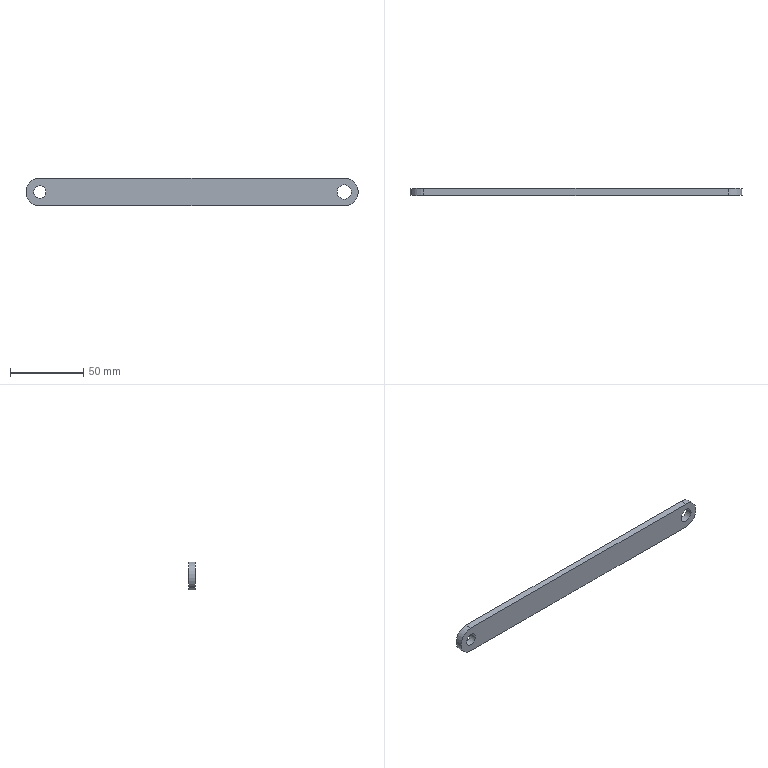Part | NX | features BREP 1 | 1 solid | 10 faces | box 227.013 x 4.763 x 19.05 mm | volume 19604 mm3 | cylinder 6 | plane 4 | commonest cylinder face diameters 8.382 x2 9.779 x2 19.05 x2
STEP:
#1=CARTESIAN_POINT('',(-103.981,0.,9.525));
#2=VERTEX_POINT('',#1);
#3=CARTESIAN_POINT('',(103.981,0.,9.525));
#4=VERTEX_POINT('',#3);
#5=CARTESIAN_POINT('',(-103.981,0.,9.525));
#6=DIRECTION('',(1.,0.,0.));
#7=VECTOR('',#6,1000.);
#8=LINE('',#5,#7);
#9=EDGE_CURVE('',#2,#4,#8,.T.);
#10=ORIENTED_EDGE('',*,*,#9,.T.);
#11=CARTESIAN_POINT('',(103.981,0.,-9.525));
#12=VERTEX_POINT('',#11);
#13=CARTESIAN_POINT('',(103.981,0.,0.));
#14=DIRECTION('',(0.,1.,0.));
#15=DIRECTION('',(0.,0.,1.));
#16=AXIS2_PLACEMENT_3D('',#13,#14,#15);
#17=CIRCLE('',#16,9.525);
#18=EDGE_CURVE('',#4,#12,#17,.T.);
#19=ORIENTED_EDGE('',*,*,#18,.T.);
#20=CARTESIAN_POINT('',(-103.981,0.,-9.525));
#21=VERTEX_POINT('',#20);
#22=CARTESIAN_POINT('',(103.981,0.,-9.525));
#23=DIRECTION('',(-1.,0.,0.));
#24=VECTOR('',#23,1000.);
#25=LINE('',#22,#24);
#26=EDGE_CURVE('',#12,#21,#25,.T.);
#27=ORIENTED_EDGE('',*,*,#26,.T.);
#28=CARTESIAN_POINT('',(-103.981,0.,0.));
#29=DIRECTION('',(0.,1.,0.));
#30=DIRECTION('',(0.,0.,-1.));
#31=AXIS2_PLACEMENT_3D('',#28,#29,#30);
#32=CIRCLE('',#31,9.525);
#33=EDGE_CURVE('',#21,#2,#32,.T.);
#34=ORIENTED_EDGE('',*,*,#33,.T.);
#35=EDGE_LOOP('',(#10,#19,#27,#34));
#36=FACE_BOUND('',#35,.T.);
#37=CARTESIAN_POINT('',(99.092,0.,0.));
#38=VERTEX_POINT('',#37);
#39=CARTESIAN_POINT('',(108.871,0.,0.));
#40=VERTEX_POINT('',#39);
#41=CARTESIAN_POINT('',(103.981,0.,0.));
#42=DIRECTION('',(0.,-1.,0.));
#43=DIRECTION('',(-1.,0.,0.));
#44=AXIS2_PLACEMENT_3D('',#41,#42,#43);
#45=CIRCLE('',#44,4.89);
#46=EDGE_CURVE('',#38,#40,#45,.T.);
#47=ORIENTED_EDGE('',*,*,#46,.T.);
#48=CARTESIAN_POINT('',(103.981,0.,0.));
#49=DIRECTION('',(0.,-1.,0.));
#50=DIRECTION('',(1.,0.,0.));
#51=AXIS2_PLACEMENT_3D('',#48,#49,#50);
#52=CIRCLE('',#51,4.89);
#53=EDGE_CURVE('',#40,#38,#52,.T.);
#54=ORIENTED_EDGE('',*,*,#53,.T.);
#55=EDGE_LOOP('',(#47,#54));
#56=FACE_BOUND('',#55,.T.);
#57=CARTESIAN_POINT('',(-108.172,0.,0.));
#58=VERTEX_POINT('',#57);
#59=CARTESIAN_POINT('',(-99.79,0.,0.));
#60=VERTEX_POINT('',#59);
#61=CARTESIAN_POINT('',(-103.981,0.,0.));
#62=DIRECTION('',(0.,-1.,0.));
#63=DIRECTION('',(-1.,0.,0.));
#64=AXIS2_PLACEMENT_3D('',#61,#62,#63);
#65=CIRCLE('',#64,4.191);
#66=EDGE_CURVE('',#58,#60,#65,.T.);
#67=ORIENTED_EDGE('',*,*,#66,.T.);
#68=CARTESIAN_POINT('',(-103.981,0.,0.));
#69=DIRECTION('',(0.,-1.,0.));
#70=DIRECTION('',(1.,0.,0.));
#71=AXIS2_PLACEMENT_3D('',#68,#69,#70);
#72=CIRCLE('',#71,4.191);
#73=EDGE_CURVE('',#60,#58,#72,.T.);
#74=ORIENTED_EDGE('',*,*,#73,.T.);
#75=EDGE_LOOP('',(#67,#74));
#76=FACE_BOUND('',#75,.T.);
#77=CARTESIAN_POINT('',(0.,0.,0.));
#78=DIRECTION('',(0.,1.,0.));
#79=DIRECTION('',(1.,0.,0.));
#80=AXIS2_PLACEMENT_3D('',#77,#78,#79);
#81=PLANE('',#80);
#82=ADVANCED_FACE('',(#36,#56,#76),#81,.T.);
#83=CARTESIAN_POINT('',(-103.981,-4.763,-9.525));
#84=VERTEX_POINT('',#83);
#85=CARTESIAN_POINT('',(-103.981,0.,-9.525));
#86=DIRECTION('',(0.,-1.,0.));
#87=VECTOR('',#86,1000.);
#88=LINE('',#85,#87);
#89=EDGE_CURVE('',#21,#84,#88,.T.);
#90=ORIENTED_EDGE('',*,*,#89,.T.);
#91=CARTESIAN_POINT('',(-103.981,-4.763,9.525));
#92=VERTEX_POINT('',#91);
#93=CARTESIAN_POINT('',(-103.981,-4.763,0.));
#94=DIRECTION('',(0.,1.,0.));
#95=DIRECTION('',(0.,0.,-1.));
#96=AXIS2_PLACEMENT_3D('',#93,#94,#95);
#97=CIRCLE('',#96,9.525);
#98=EDGE_CURVE('',#84,#92,#97,.T.);
#99=ORIENTED_EDGE('',*,*,#98,.T.);
#100=CARTESIAN_POINT('',(-103.981,0.,9.525));
#101=DIRECTION('',(0.,-1.,0.));
#102=VECTOR('',#101,1000.);
#103=LINE('',#100,#102);
#104=EDGE_CURVE('',#2,#92,#103,.T.);
#105=ORIENTED_EDGE('',*,*,#104,.F.);
#106=ORIENTED_EDGE('',*,*,#33,.F.);
#107=EDGE_LOOP('',(#90,#99,#105,#106));
#108=FACE_BOUND('',#107,.T.);
#109=CARTESIAN_POINT('',(-103.981,-2.381,0.));
#110=DIRECTION('',(0.,1.,0.));
#111=DIRECTION('',(0.,0.,-1.));
#112=AXIS2_PLACEMENT_3D('',#109,#110,#111);
#113=CYLINDRICAL_SURFACE('',#112,9.525);
#114=ADVANCED_FACE('',(#108),#113,.T.);
#115=ORIENTED_EDGE('',*,*,#104,.T.);
#116=CARTESIAN_POINT('',(103.981,-4.763,9.525));
#117=VERTEX_POINT('',#116);
#118=CARTESIAN_POINT('',(-103.981,-4.763,9.525));
#119=DIRECTION('',(1.,0.,0.));
#120=VECTOR('',#119,1000.);
#121=LINE('',#118,#120);
#122=EDGE_CURVE('',#92,#117,#121,.T.);
#123=ORIENTED_EDGE('',*,*,#122,.T.);
#124=CARTESIAN_POINT('',(103.981,0.,9.525));
#125=DIRECTION('',(0.,-1.,0.));
#126=VECTOR('',#125,1000.);
#127=LINE('',#124,#126);
#128=EDGE_CURVE('',#4,#117,#127,.T.);
#129=ORIENTED_EDGE('',*,*,#128,.F.);
#130=ORIENTED_EDGE('',*,*,#9,.F.);
#131=EDGE_LOOP('',(#115,#123,#129,#130));
#132=FACE_BOUND('',#131,.T.);
#133=CARTESIAN_POINT('',(0.,-2.381,9.525));
#134=DIRECTION('',(0.,0.,1.));
#135=DIRECTION('',(1.,0.,0.));
#136=AXIS2_PLACEMENT_3D('',#133,#134,#135);
#137=PLANE('',#136);
#138=ADVANCED_FACE('',(#132),#137,.T.);
#139=ORIENTED_EDGE('',*,*,#128,.T.);
#140=CARTESIAN_POINT('',(103.981,-4.763,-9.525));
#141=VERTEX_POINT('',#140);
#142=CARTESIAN_POINT('',(103.981,-4.763,0.));
#143=DIRECTION('',(0.,1.,0.));
#144=DIRECTION('',(0.,0.,1.));
#145=AXIS2_PLACEMENT_3D('',#142,#143,#144);
#146=CIRCLE('',#145,9.525);
#147=EDGE_CURVE('',#117,#141,#146,.T.);
#148=ORIENTED_EDGE('',*,*,#147,.T.);
#149=CARTESIAN_POINT('',(103.981,0.,-9.525));
#150=DIRECTION('',(0.,-1.,0.));
#151=VECTOR('',#150,1000.);
#152=LINE('',#149,#151);
#153=EDGE_CURVE('',#12,#141,#152,.T.);
#154=ORIENTED_EDGE('',*,*,#153,.F.);
#155=ORIENTED_EDGE('',*,*,#18,.F.);
#156=EDGE_LOOP('',(#139,#148,#154,#155));
#157=FACE_BOUND('',#156,.T.);
#158=CARTESIAN_POINT('',(103.981,-2.381,0.));
#159=DIRECTION('',(0.,1.,0.));
#160=DIRECTION('',(0.,0.,1.));
#161=AXIS2_PLACEMENT_3D('',#158,#159,#160);
#162=CYLINDRICAL_SURFACE('',#161,9.525);
#163=ADVANCED_FACE('',(#157),#162,.T.);
#164=ORIENTED_EDGE('',*,*,#153,.T.);
#165=CARTESIAN_POINT('',(103.981,-4.763,-9.525));
#166=DIRECTION('',(-1.,0.,0.));
#167=VECTOR('',#166,1000.);
#168=LINE('',#165,#167);
#169=EDGE_CURVE('',#141,#84,#168,.T.);
#170=ORIENTED_EDGE('',*,*,#169,.T.);
#171=ORIENTED_EDGE('',*,*,#89,.F.);
#172=ORIENTED_EDGE('',*,*,#26,.F.);
#173=EDGE_LOOP('',(#164,#170,#171,#172));
#174=FACE_BOUND('',#173,.T.);
#175=CARTESIAN_POINT('',(0.,-2.381,-9.525));
#176=DIRECTION('',(0.,0.,-1.));
#177=DIRECTION('',(0.,-1.,0.));
#178=AXIS2_PLACEMENT_3D('',#175,#176,#177);
#179=PLANE('',#178);
#180=ADVANCED_FACE('',(#174),#179,.T.);
#181=ORIENTED_EDGE('',*,*,#169,.F.);
#182=ORIENTED_EDGE('',*,*,#147,.F.);
#183=ORIENTED_EDGE('',*,*,#122,.F.);
#184=ORIENTED_EDGE('',*,*,#98,.F.);
#185=EDGE_LOOP('',(#181,#182,#183,#184));
#186=FACE_BOUND('',#185,.T.);
#187=CARTESIAN_POINT('',(99.092,-4.763,0.));
#188=VERTEX_POINT('',#187);
#189=CARTESIAN_POINT('',(108.871,-4.763,0.));
#190=VERTEX_POINT('',#189);
#191=CARTESIAN_POINT('',(103.981,-4.763,0.));
#192=DIRECTION('',(0.,-1.,0.));
#193=DIRECTION('',(-1.,0.,0.));
#194=AXIS2_PLACEMENT_3D('',#191,#192,#193);
#195=CIRCLE('',#194,4.89);
#196=EDGE_CURVE('',#188,#190,#195,.T.);
#197=ORIENTED_EDGE('',*,*,#196,.F.);
#198=CARTESIAN_POINT('',(103.981,-4.763,0.));
#199=DIRECTION('',(0.,-1.,0.));
#200=DIRECTION('',(1.,0.,0.));
#201=AXIS2_PLACEMENT_3D('',#198,#199,#200);
#202=CIRCLE('',#201,4.89);
#203=EDGE_CURVE('',#190,#188,#202,.T.);
#204=ORIENTED_EDGE('',*,*,#203,.F.);
#205=EDGE_LOOP('',(#197,#204));
#206=FACE_BOUND('',#205,.T.);
#207=CARTESIAN_POINT('',(-108.172,-4.763,0.));
#208=VERTEX_POINT('',#207);
#209=CARTESIAN_POINT('',(-99.79,-4.763,0.));
#210=VERTEX_POINT('',#209);
#211=CARTESIAN_POINT('',(-103.981,-4.763,0.));
#212=DIRECTION('',(0.,-1.,0.));
#213=DIRECTION('',(-1.,0.,0.));
#214=AXIS2_PLACEMENT_3D('',#211,#212,#213);
#215=CIRCLE('',#214,4.191);
#216=EDGE_CURVE('',#208,#210,#215,.T.);
#217=ORIENTED_EDGE('',*,*,#216,.F.);
#218=CARTESIAN_POINT('',(-103.981,-4.763,0.));
#219=DIRECTION('',(0.,-1.,0.));
#220=DIRECTION('',(1.,0.,0.));
#221=AXIS2_PLACEMENT_3D('',#218,#219,#220);
#222=CIRCLE('',#221,4.191);
#223=EDGE_CURVE('',#210,#208,#222,.T.);
#224=ORIENTED_EDGE('',*,*,#223,.F.);
#225=EDGE_LOOP('',(#217,#224));
#226=FACE_BOUND('',#225,.T.);
#227=CARTESIAN_POINT('',(0.,-4.763,0.));
#228=DIRECTION('',(0.,1.,0.));
#229=DIRECTION('',(1.,0.,0.));
#230=AXIS2_PLACEMENT_3D('',#227,#228,#229);
#231=PLANE('',#230);
#232=ADVANCED_FACE('',(#186,#206,#226),#231,.F.);
#233=CARTESIAN_POINT('',(108.871,0.,0.));
#234=DIRECTION('',(0.,-1.,0.));
#235=VECTOR('',#234,1000.);
#236=LINE('',#233,#235);
#237=EDGE_CURVE('',#190,#40,#236,.F.);
#238=ORIENTED_EDGE('',*,*,#237,.F.);
#239=ORIENTED_EDGE('',*,*,#203,.T.);
#240=CARTESIAN_POINT('',(99.092,0.,0.));
#241=DIRECTION('',(0.,-1.,0.));
#242=VECTOR('',#241,1000.);
#243=LINE('',#240,#242);
#244=EDGE_CURVE('',#188,#38,#243,.F.);
#245=ORIENTED_EDGE('',*,*,#244,.T.);
#246=ORIENTED_EDGE('',*,*,#53,.F.);
#247=EDGE_LOOP('',(#238,#239,#245,#246));
#248=FACE_BOUND('',#247,.T.);
#249=CARTESIAN_POINT('',(103.981,0.,0.));
#250=DIRECTION('',(0.,-1.,0.));
#251=DIRECTION('',(1.,0.,0.));
#252=AXIS2_PLACEMENT_3D('',#249,#250,#251);
#253=CYLINDRICAL_SURFACE('',#252,4.89);
#254=ADVANCED_FACE('',(#248),#253,.F.);
#255=ORIENTED_EDGE('',*,*,#244,.F.);
#256=ORIENTED_EDGE('',*,*,#196,.T.);
#257=ORIENTED_EDGE('',*,*,#237,.T.);
#258=ORIENTED_EDGE('',*,*,#46,.F.);
#259=EDGE_LOOP('',(#255,#256,#257,#258));
#260=FACE_BOUND('',#259,.T.);
#261=CARTESIAN_POINT('',(103.981,0.,0.));
#262=DIRECTION('',(0.,-1.,0.));
#263=DIRECTION('',(1.,0.,0.));
#264=AXIS2_PLACEMENT_3D('',#261,#262,#263);
#265=CYLINDRICAL_SURFACE('',#264,4.89);
#266=ADVANCED_FACE('',(#260),#265,.F.);
#267=CARTESIAN_POINT('',(-99.79,0.,0.));
#268=DIRECTION('',(0.,-1.,0.));
#269=VECTOR('',#268,1000.);
#270=LINE('',#267,#269);
#271=EDGE_CURVE('',#210,#60,#270,.F.);
#272=ORIENTED_EDGE('',*,*,#271,.F.);
#273=ORIENTED_EDGE('',*,*,#223,.T.);
#274=CARTESIAN_POINT('',(-108.172,0.,0.));
#275=DIRECTION('',(0.,-1.,0.));
#276=VECTOR('',#275,1000.);
#277=LINE('',#274,#276);
#278=EDGE_CURVE('',#208,#58,#277,.F.);
#279=ORIENTED_EDGE('',*,*,#278,.T.);
#280=ORIENTED_EDGE('',*,*,#73,.F.);
#281=EDGE_LOOP('',(#272,#273,#279,#280));
#282=FACE_BOUND('',#281,.T.);
#283=CARTESIAN_POINT('',(-103.981,0.,0.));
#284=DIRECTION('',(0.,-1.,0.));
#285=DIRECTION('',(1.,0.,0.));
#286=AXIS2_PLACEMENT_3D('',#283,#284,#285);
#287=CYLINDRICAL_SURFACE('',#286,4.191);
#288=ADVANCED_FACE('',(#282),#287,.F.);
#289=ORIENTED_EDGE('',*,*,#278,.F.);
#290=ORIENTED_EDGE('',*,*,#216,.T.);
#291=ORIENTED_EDGE('',*,*,#271,.T.);
#292=ORIENTED_EDGE('',*,*,#66,.F.);
#293=EDGE_LOOP('',(#289,#290,#291,#292));
#294=FACE_BOUND('',#293,.T.);
#295=CARTESIAN_POINT('',(-103.981,0.,0.));
#296=DIRECTION('',(0.,-1.,0.));
#297=DIRECTION('',(1.,0.,0.));
#298=AXIS2_PLACEMENT_3D('',#295,#296,#297);
#299=CYLINDRICAL_SURFACE('',#298,4.191);
#300=ADVANCED_FACE('',(#294),#299,.F.);
#301=CLOSED_SHELL('',(#82,#114,#138,#163,#180,#232,#254,#266,#288,#300));
#302=MANIFOLD_SOLID_BREP('',#301);
#303=(LENGTH_UNIT()NAMED_UNIT(*)SI_UNIT(.MILLI.,.METRE.));
#304=UNCERTAINTY_MEASURE_WITH_UNIT(LENGTH_MEASURE(0.00001),#303,'','');
#305=(NAMED_UNIT(*)PLANE_ANGLE_UNIT()SI_UNIT($,.RADIAN.));
#306=(NAMED_UNIT(*)SI_UNIT($,.STERADIAN.)SOLID_ANGLE_UNIT());
#307=(GEOMETRIC_REPRESENTATION_CONTEXT(3)GLOBAL_UNCERTAINTY_ASSIGNED_CONTEXT((#304))GLOBAL_UNIT_ASSIGNED_CONTEXT((#303,#305,#306))REPRESENTATION_CONTEXT('',''));
#308=ADVANCED_BREP_SHAPE_REPRESENTATION('',(#302),#307);